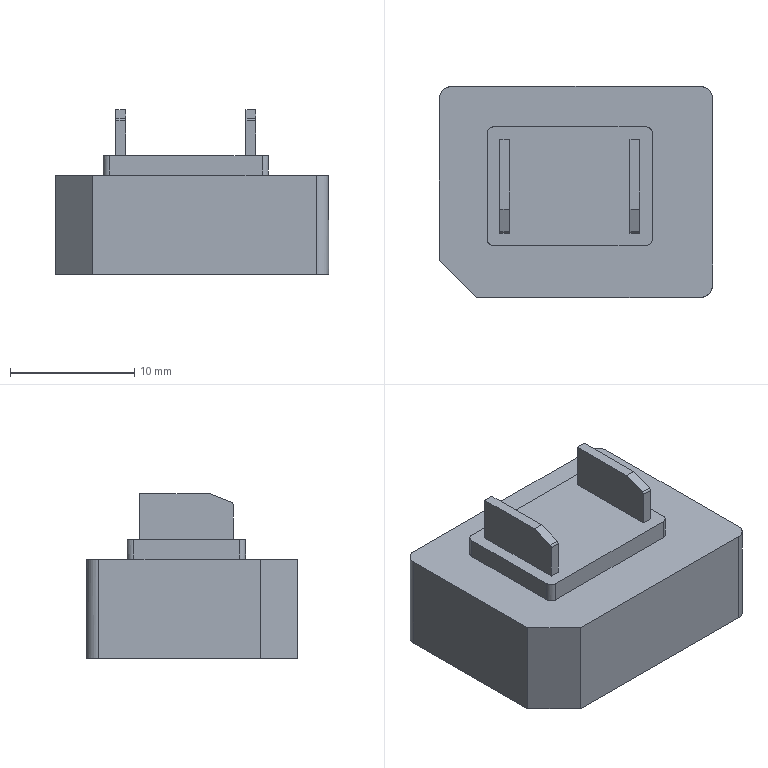NC program | PowerMill | posted by the shop | part box 22 x 17 x 13.286 mm
Lines 8691 to 10398 of 53717:
( TOOL ID   D3_1_1 )
( TOOL DIA. 3. TIP RAD 0 LENGTH 59.04 )
( Z = -3.934 )
T10 M6
T13
G91 G28 Z0
G0 G90 G54
M08
S18000 M3
X0 Y0 M8
G43 Z10.795 H10
X6.194 Y-3.121
Z1.037
G1 Z-.163 F960
X6.18 Y-3.08 F1600
X6.161 Y-3.04
X6.14 Y-3.002
X6.115 Y-2.966
X6.086 Y-2.932
X6.055 Y-2.902
X6.021 Y-2.874
X5.985 Y-2.849
X5.947 Y-2.828
X5.907 Y-2.811
X5.865 Y-2.797
X5.823 Y-2.787
X5.779 Y-2.781
X5.736 Y-2.779
X5.692 Y-2.78
X5.649 Y-2.786
X5.606 Y-2.796
X5.596 Y-2.799
X5.519 Y-2.822
X5.445 Y-2.84
X5.375 Y-2.854
X5.309 Y-2.863
X5.244 Y-2.868
X5.182 Y-2.87
X4.846 Y-2.871
X4.548 Y-2.87
X4.399 Y-2.871
X4.313 Y-2.87
X4.232 Y-2.866
X4.154 Y-2.858
X4.081 Y-2.846
X4.01 Y-2.832
X3.941 Y-2.813
X3.868 Y-2.79
X3.797 Y-2.763
X3.728 Y-2.733
X3.66 Y-2.699
X3.595 Y-2.661
X3.531 Y-2.62
X3.469 Y-2.575
X3.41 Y-2.528
X3.353 Y-2.477
X3.299 Y-2.424
X3.248 Y-2.367
X3.2 Y-2.308
X3.155 Y-2.247
X3.114 Y-2.183
X3.076 Y-2.118
X3.041 Y-2.05
X3.01 Y-1.981
X2.983 Y-1.911
X2.96 Y-1.84
X2.94 Y-1.768
X2.925 Y-1.695
X2.912 Y-1.62
X2.904 Y-1.544
X2.9 Y-1.466
X2.899 Y-1.393
X2.902 Y-1.317
X2.908 Y-1.241
X2.919 Y-1.165
X2.934 Y-1.09
X2.952 Y-1.017
X2.975 Y-.944
X3.001 Y-.872
X3.031 Y-.802
X3.064 Y-.734
X3.101 Y-.668
X3.141 Y-.604
X3.185 Y-.542
X3.231 Y-.483
X3.281 Y-.426
X3.334 Y-.372
X3.39 Y-.32
X3.449 Y-.271
X3.51 Y-.225
X3.572 Y-.183
X3.637 Y-.145
X3.704 Y-.11
X3.773 Y-.077
X3.844 Y-.049
X3.916 Y-.025
X3.988 Y-.004
X4.061 Y.012
X4.134 Y.025
X4.207 Y.033
X4.281 Y.038
X4.354 Y.039
X4.54 Y.04
X4.873
X5.099
X5.173 Y.039
X5.251 Y.035
X5.327 Y.028
X5.399 Y.018
X5.47 Y.004
X5.538 Y-.013
X5.607 Y-.034
X5.676 Y-.06
X5.745 Y-.089
X5.814 Y-.123
X5.881 Y-.16
X5.946 Y-.201
X6.009 Y-.245
X6.069 Y-.291
X6.126 Y-.34
X6.179 Y-.391
X6.228 Y-.445
X6.277 Y-.503
X6.323 Y-.564
X6.365 Y-.627
X6.405 Y-.692
X6.44 Y-.759
X6.473 Y-.828
X6.501 Y-.899
X6.526 Y-.971
X6.547 Y-1.044
X6.564 Y-1.119
X6.578 Y-1.194
X6.587 Y-1.27
X6.592 Y-1.346
X6.594 Y-1.422
X6.591 Y-1.5
X6.585 Y-1.578
X6.575 Y-1.654
X6.561 Y-1.729
X6.543 Y-1.803
X6.521 Y-1.876
X6.495 Y-1.948
X6.466 Y-2.017
X6.434 Y-2.085
X6.397 Y-2.152
X6.358 Y-2.216
X6.314 Y-2.279
X6.268 Y-2.339
X6.219 Y-2.396
X6.166 Y-2.451
X6.111 Y-2.503
X6.053 Y-2.552
X5.993 Y-2.598
X5.93 Y-2.641
X5.865 Y-2.68
X5.799 Y-2.716
X5.73 Y-2.748
X5.66 Y-2.776
X5.596 Y-2.799
X5.556 Y-2.815
X5.517 Y-2.835
X5.48 Y-2.859
X5.445 Y-2.885
X5.413 Y-2.915
X5.384 Y-2.948
X5.358 Y-2.983
X5.335 Y-3.02
X5.315 Y-3.059
X5.3 Y-3.1
X5.288 Y-3.142
X5.28 Y-3.185
X5.276 Y-3.229
X5.275 Y-3.272
X5.279 Y-3.316
X5.287 Y-3.359
X5.299 Y-3.401
X5.302 Y-3.41
X6.224 Y-3.172 Z-.193
X6.209 Y-3.131
X6.19 Y-3.092
X6.167 Y-3.055
X6.141 Y-3.019
X6.112 Y-2.987
X6.08 Y-2.957
X6.045 Y-2.93
X6.008 Y-2.906
X5.97 Y-2.886
X5.929 Y-2.87
X5.887 Y-2.857
X5.844 Y-2.848
X5.801 Y-2.843
X5.757 Y-2.842
X5.714 Y-2.845
X5.67 Y-2.852
X5.628 Y-2.863
X5.619 Y-2.866
X5.568 Y-2.883
X5.51 Y-2.899
X5.459 Y-2.911
X5.406 Y-2.922
X5.354 Y-2.93
X5.278 Y-2.938
X5.195 Y-2.944
X5.104 Y-2.945
X5.005
X4.637
X4.399 Y-2.946
X4.316 Y-2.945
X4.235 Y-2.941
X4.156 Y-2.933
X4.08 Y-2.921
X4.006 Y-2.905
X3.934 Y-2.886
X3.863 Y-2.863
X3.794 Y-2.837
X3.727 Y-2.807
X3.661 Y-2.774
X3.595 Y-2.736
X3.53 Y-2.694
X3.468 Y-2.65
X3.409 Y-2.602
X3.352 Y-2.551
X3.299 Y-2.498
X3.248 Y-2.442
X3.201 Y-2.384
X3.156 Y-2.322
X3.114 Y-2.259
X3.076 Y-2.193
X3.042 Y-2.126
X3.011 Y-2.058
X2.988 Y-1.998
X2.967 Y-1.937
X2.948 Y-1.875
X2.933 Y-1.811
X2.92 Y-1.742
X2.91 Y-1.669
X2.903 Y-1.592
X2.9 Y-1.515
X2.899 Y-1.441
X2.9 Y-1.366
X2.904 Y-1.289
X2.912 Y-1.212
X2.924 Y-1.137
X2.94 Y-1.063
X2.96 Y-.99
X2.983 Y-.919
X3.01 Y-.85
X3.041 Y-.78
X3.076 Y-.712
X3.114 Y-.646
X3.156 Y-.583
X3.201 Y-.521
X3.249 Y-.463
X3.3 Y-.406
X3.354 Y-.353
X3.41 Y-.302
X3.47 Y-.255
X3.531 Y-.21
X3.595 Y-.169
X3.661 Y-.131
X3.729 Y-.097
X3.799 Y-.067
X3.87 Y-.04
X3.942 Y-.017
X4.007 Y0
X4.082 Y.016
X4.153 Y.028
X4.22 Y.035
X4.284 Y.039
X4.347
X4.699 Y.04
X4.921 Y.041
X5.096
X5.198 Y.039
X5.27 Y.035
X5.342 Y.027
X5.415 Y.016
X5.488 Y0
X5.561 Y-.02
X5.633 Y-.044
X5.706 Y-.073
X5.774 Y-.103
X5.84 Y-.137
X5.905 Y-.174
X5.968 Y-.215
X6.029 Y-.26
X6.088 Y-.308
X6.145 Y-.359
X6.198 Y-.412
X6.248 Y-.468
X6.296 Y-.527
X6.34 Y-.588
X6.381 Y-.652
X6.419 Y-.718
X6.454 Y-.787
X6.485 Y-.857
X6.511 Y-.926
X6.534 Y-.996
X6.553 Y-1.068
X6.569 Y-1.142
X6.581 Y-1.218
X6.589 Y-1.295
X6.593 Y-1.373
X6.594 Y-1.443
X6.593 Y-1.514
X6.59 Y-1.586
X6.584 Y-1.661
X6.575 Y-1.733
X6.562 Y-1.801
X6.547 Y-1.864
X6.53 Y-1.924
X6.51 Y-1.984
X6.487 Y-2.044
X6.457 Y-2.113
X6.423 Y-2.181
X6.386 Y-2.246
X6.345 Y-2.31
X6.301 Y-2.372
X6.253 Y-2.431
X6.203 Y-2.488
X6.149 Y-2.542
X6.093 Y-2.593
X6.034 Y-2.642
X5.973 Y-2.687
X5.909 Y-2.729
X5.844 Y-2.767
X5.777 Y-2.802
X5.708 Y-2.832
X5.639 Y-2.86
X5.619 Y-2.866
X5.578 Y-2.882
X5.538 Y-2.901
X5.501 Y-2.924
X5.466 Y-2.95
X5.433 Y-2.979
X5.403 Y-3.011
X5.376 Y-3.045
X5.353 Y-3.082
X5.333 Y-3.121
X5.316 Y-3.162
X5.303 Y-3.203
X5.295 Y-3.246
X5.29 Y-3.29
X5.289 Y-3.333
X5.292 Y-3.377
X5.299 Y-3.42
X5.309 Y-3.463
X5.312 Y-3.472
X6.265 Y-3.206 Z-.223
X6.248 Y-3.166
X6.226 Y-3.128
X6.202 Y-3.092
X6.174 Y-3.058
X6.143 Y-3.027
X6.11 Y-2.999
X6.074 Y-2.974
X6.036 Y-2.952
X5.996 Y-2.934
X5.954 Y-2.92
X5.912 Y-2.909
X5.869 Y-2.902
X5.825 Y-2.9
X5.781 Y-2.901
X5.738 Y-2.906
X5.695 Y-2.916
X5.653 Y-2.929
X5.644 Y-2.932
X5.635 Y-2.936
X5.562 Y-2.96
X5.489 Y-2.979
X5.415 Y-2.995
X5.394 Y-2.999
X5.323 Y-3.009
X5.248 Y-3.016
X5.168 Y-3.02
X5.08
X4.878
X4.612
X4.417
X4.326
X4.246 Y-3.017
X4.173 Y-3.01
X4.106 Y-3.001
X4.04 Y-2.988
X3.965 Y-2.969
X3.892 Y-2.947
X3.821 Y-2.922
X3.751 Y-2.893
X3.683 Y-2.86
X3.616 Y-2.823
X3.552 Y-2.783
X3.489 Y-2.74
X3.429 Y-2.694
X3.372 Y-2.644
X3.317 Y-2.591
X3.265 Y-2.536
X3.216 Y-2.478
X3.17 Y-2.417
X3.127 Y-2.354
X3.088 Y-2.289
X3.052 Y-2.222
X3.02 Y-2.154
X2.991 Y-2.083
X2.966 Y-2.011
X2.945 Y-1.938
X2.928 Y-1.865
X2.915 Y-1.791
X2.906 Y-1.716
X2.901 Y-1.642
X2.899 Y-1.567
Y-1.393
X2.902 Y-1.317
X2.908 Y-1.242
X2.919 Y-1.166
X2.933 Y-1.092
X2.952 Y-1.018
X2.974 Y-.946
X3. Y-.875
X3.03 Y-.805
X3.063 Y-.736
X3.1 Y-.67
X3.14 Y-.606
X3.184 Y-.544
X3.231 Y-.484
X3.28 Y-.427
X3.333 Y-.372
X3.389 Y-.321
X3.447 Y-.272
X3.508 Y-.227
X3.571 Y-.184
X3.636 Y-.145
X3.703 Y-.11
X3.772 Y-.078
X3.843 Y-.05
X3.915 Y-.025
X3.988 Y-.005
X4.055 Y.011
X4.123 Y.023
X4.193 Y.031
X4.27 Y.037
X4.347 Y.04
X4.421
X4.799
X5.021
X5.173 Y.039
X5.247 Y.036
X5.32 Y.03
X5.394 Y.019
X5.467 Y.005
X5.54 Y-.014
X5.612 Y-.036
X5.683 Y-.063
X5.753 Y-.093
X5.822 Y-.127
X5.888 Y-.164
X5.952 Y-.204
X6.014 Y-.248
X6.074 Y-.295
X6.131 Y-.346
X6.185 Y-.399
X6.236 Y-.455
X6.285 Y-.513
X6.33 Y-.574
X6.372 Y-.637
X6.411 Y-.703
X6.446 Y-.77
X6.478 Y-.839
X6.506 Y-.91
X6.53 Y-.982
X6.55 Y-1.055
X6.567 Y-1.129
X6.579 Y-1.204
X6.588 Y-1.28
X6.592 Y-1.355
X6.593 Y-1.423
X6.594 Y-1.491
X6.593 Y-1.565
X6.591 Y-1.648
X6.586 Y-1.722
X6.578 Y-1.787
X6.568 Y-1.846
X6.556 Y-1.903
X6.541 Y-1.96
X6.524 Y-2.016
X6.504 Y-2.072
X6.483 Y-2.127
X6.454 Y-2.194
X6.421 Y-2.26
X6.384 Y-2.325
X6.343 Y-2.388
X6.299 Y-2.449
X6.251 Y-2.509
X6.2 Y-2.566
X6.147 Y-2.619
X6.091 Y-2.67
X6.033 Y-2.718
X5.972 Y-2.762
X5.908 Y-2.804
X5.843 Y-2.842
X5.775 Y-2.877
X5.706 Y-2.908
X5.644 Y-2.932
X5.604 Y-2.95
X5.566 Y-2.971
X5.53 Y-2.996
X5.496 Y-3.023
X5.465 Y-3.054
X5.437 Y-3.088
X5.412 Y-3.124
X5.39 Y-3.162
X5.372 Y-3.202
X5.358 Y-3.243
X5.347 Y-3.285
X5.34 Y-3.329
X5.338 Y-3.372
X5.339 Y-3.416
X5.344 Y-3.459
X5.354 Y-3.502
X5.367 Y-3.544
X5.37 Y-3.553
X6.291 Y-3.27 Z-.252
X6.274 Y-3.23
X6.252 Y-3.192
X6.228 Y-3.155
X6.2 Y-3.122
X6.169 Y-3.091
X6.135 Y-3.063
X6.099 Y-3.038
X6.061 Y-3.016
X6.021 Y-2.998
X5.98 Y-2.984
X5.937 Y-2.974
X5.894 Y-2.967
X5.85 Y-2.965
X5.807 Y-2.966
X5.763 Y-2.971
X5.721 Y-2.981
X5.679 Y-2.994
X5.67 Y-2.997
X5.665 Y-2.999
X5.59 Y-3.026
X5.517 Y-3.048
X5.445 Y-3.065
X5.376 Y-3.079
X5.308 Y-3.088
X5.242 Y-3.093
X5.176 Y-3.094
X4.849 Y-3.095
X4.572
X4.399 Y-3.096
X4.317 Y-3.095
X4.237 Y-3.091
X4.16 Y-3.083
X4.085 Y-3.072
X4.012 Y-3.057
X3.942 Y-3.038
X3.872 Y-3.016
X3.804 Y-2.99
X3.734 Y-2.96
X3.666 Y-2.926
X3.6 Y-2.889
X3.536 Y-2.848
X3.474 Y-2.804
X3.415 Y-2.757
X3.358 Y-2.706
X3.304 Y-2.653
X3.253 Y-2.597
X3.204 Y-2.538
X3.159 Y-2.477
X3.117 Y-2.414
X3.079 Y-2.349
X3.044 Y-2.281
X3.013 Y-2.212
X2.985 Y-2.141
X2.961 Y-2.069
X2.941 Y-1.996
X2.925 Y-1.922
X2.913 Y-1.847
X2.904 Y-1.772
X2.9 Y-1.696
X2.899 Y-1.621
Y-1.411
X2.901 Y-1.335
X2.907 Y-1.259
X2.916 Y-1.184
X2.93 Y-1.109
X2.947 Y-1.035
X2.969 Y-.962
X2.994 Y-.89
X3.023 Y-.82
X3.055 Y-.751
X3.092 Y-.685
X3.131 Y-.62
X3.174 Y-.557
X3.22 Y-.497
X3.269 Y-.439
X3.322 Y-.384
X3.377 Y-.332
X3.434 Y-.282
X3.495 Y-.236
X3.557 Y-.193
X3.622 Y-.153
X3.689 Y-.117
X3.758 Y-.085
X3.828 Y-.056
X3.899 Y-.03
X3.972 Y-.009
X4.039 Y.007
X4.106 Y.02
X4.174 Y.029
X4.249 Y.036
X4.328 Y.039
X4.399 Y.04
X4.799
X5. Y.041
X5.14 Y.04
X5.214 Y.039
X5.287 Y.033
X5.361 Y.024
X5.435 Y.011
X5.508 Y-.006
X5.581 Y-.027
X5.653 Y-.052
X5.725 Y-.08
X5.793 Y-.112
X5.86 Y-.147
X5.924 Y-.186
X5.987 Y-.228
X6.048 Y-.274
X6.106 Y-.323
X6.161 Y-.375
X6.214 Y-.429
X6.264 Y-.487
X6.31 Y-.546
X6.354 Y-.609
X6.394 Y-.673
X6.431 Y-.74
X6.464 Y-.808
X6.494 Y-.878
X6.519 Y-.95
X6.542 Y-1.022
X6.56 Y-1.096
X6.574 Y-1.17
X6.584 Y-1.246
X6.591 Y-1.321
X6.593 Y-1.397
Y-1.473
Y-1.633
X6.591 Y-1.706
X6.587 Y-1.78
X6.579 Y-1.854
X6.566 Y-1.927
X6.55 Y-2.
X6.53 Y-2.073
X6.506 Y-2.144
X6.478 Y-2.215
X6.446 Y-2.285
X6.411 Y-2.352
X6.373 Y-2.417
X6.331 Y-2.48
X6.286 Y-2.541
X6.237 Y-2.599
X6.186 Y-2.655
X6.132 Y-2.709
X6.075 Y-2.759
X6.015 Y-2.806
X5.953 Y-2.85
X5.889 Y-2.89
X5.823 Y-2.928
X5.755 Y-2.961
X5.686 Y-2.991
X5.67 Y-2.997
X5.63 Y-3.015
X5.591 Y-3.036
X5.555 Y-3.061
X5.522 Y-3.089
X5.491 Y-3.12
X5.463 Y-3.154
X5.438 Y-3.19
X5.416 Y-3.228
X5.398 Y-3.268
X5.384 Y-3.309
X5.373 Y-3.351
X5.367 Y-3.395
X5.364 Y-3.438
X5.366 Y-3.482
X5.371 Y-3.526
X5.381 Y-3.568
X5.394 Y-3.61
X5.397 Y-3.619
X6.326 Y-3.316 Z-.282
X6.307 Y-3.277
X6.284 Y-3.239
X6.259 Y-3.204
X6.23 Y-3.171
X6.198 Y-3.141
X6.164 Y-3.113
X6.127 Y-3.09
X6.088 Y-3.069
X6.048 Y-3.052
X6.006 Y-3.039
X5.964 Y-3.03
X5.92 Y-3.025
X5.876 Y-3.023
X5.833 Y-3.026
X5.789 Y-3.032
X5.747 Y-3.043
X5.706 Y-3.057
X5.697 Y-3.061
X5.678 Y-3.069
X5.607 Y-3.095
X5.595 Y-3.099
X5.517 Y-3.122
X5.443 Y-3.14
X5.373 Y-3.154
X5.307 Y-3.163
X5.243 Y-3.168
X5.18 Y-3.169
X4.845 Y-3.17
X4.52
X4.399
X4.31 Y-3.169
X4.23 Y-3.165
X4.157 Y-3.158
X4.088 Y-3.147
X4.013 Y-3.131
X3.939 Y-3.112
X3.866 Y-3.089
X3.795 Y-3.062
X3.726 Y-3.031
X3.659 Y-2.997
X3.593 Y-2.959
X3.529 Y-2.918
X3.468 Y-2.874
X3.409 Y-2.826
X3.352 Y-2.775
X3.298 Y-2.722
X3.247 Y-2.666
X3.199 Y-2.607
X3.155 Y-2.545
X3.113 Y-2.482
X3.075 Y-2.416
X3.041 Y-2.349
X3.01 Y-2.279
X2.982 Y-2.208
X2.959 Y-2.136
X2.939 Y-2.063
X2.923 Y-1.989
X2.912 Y-1.915
X2.904 Y-1.84
X2.9 Y-1.765
X2.899 Y-1.69
Y-1.193
Y-.349
Y2.899
Y4.199
X2.901 Y4.285
X2.906 Y4.363
X2.914 Y4.435
X2.925 Y4.502
X2.942 Y4.577
X2.962 Y4.651
X2.986 Y4.723
X3.014 Y4.794
X3.046 Y4.863
X3.081 Y4.931
X3.12 Y4.996
X3.162 Y5.06
X3.207 Y5.121
X3.255 Y5.179
X3.307 Y5.235
X3.361 Y5.288
X3.417 Y5.338
X3.476 Y5.384
X3.538 Y5.428
X3.603 Y5.469
X3.669 Y5.506
X3.737 Y5.54
X3.806 Y5.57
X3.877 Y5.596
X3.948 Y5.619
X4.021 Y5.638
X4.094 Y5.652
X4.167 Y5.663
X4.238 Y5.67
X4.31 Y5.672
X4.495 Y5.674
X4.699
X5.007
X5.099
X5.185 Y5.673
X5.265 Y5.669
X5.339 Y5.661
X5.409 Y5.65
X5.484 Y5.634
X5.557 Y5.615
X5.63 Y5.591
X5.7 Y5.564
X5.77 Y5.533
X5.837 Y5.499
X5.903 Y5.461
X5.967 Y5.419
X6.028 Y5.375
X6.087 Y5.327
X6.144 Y5.276
X6.197 Y5.222
X6.248 Y5.166
X6.296 Y5.107
X6.34 Y5.045
X6.381 Y4.982
X6.419 Y4.916
X6.454 Y4.847
X6.485 Y4.777
X6.511 Y4.709
X6.534 Y4.64
X6.552 Y4.57
X6.568 Y4.497
X6.579 Y4.422
X6.587 Y4.344
X6.592 Y4.262
X6.593 Y4.177
Y2.28
Y-1.3
X6.594 Y-1.699
X6.592 Y-1.778
X6.587 Y-1.857
X6.577 Y-1.934
X6.564 Y-2.01
X6.547 Y-2.085
X6.526 Y-2.158
X6.501 Y-2.23
X6.473 Y-2.3
X6.442 Y-2.369
X6.406 Y-2.435
X6.368 Y-2.499
X6.326 Y-2.562
X6.28 Y-2.623
X6.231 Y-2.681
X6.18 Y-2.737
X6.125 Y-2.79
X6.068 Y-2.839
X6.008 Y-2.886
X5.946 Y-2.93
X5.882 Y-2.97
X5.816 Y-3.006
X5.748 Y-3.039
X5.697 Y-3.061
X5.657 Y-3.08
X5.619 Y-3.102
X5.584 Y-3.128
X5.551 Y-3.157
X5.521 Y-3.189
X5.494 Y-3.223
X5.47 Y-3.26
X5.449 Y-3.298
X5.433 Y-3.339
X5.419 Y-3.38
X5.41 Y-3.423
X5.405 Y-3.467
X5.404 Y-3.51
X5.406 Y-3.554
X5.413 Y-3.597
X5.423 Y-3.64
X5.438 Y-3.681
X5.441 Y-3.69
X6.349 Y-3.388 Z-.312
X6.33 Y-3.348
X6.309 Y-3.31
X6.283 Y-3.275
X6.255 Y-3.241
X6.223 Y-3.211
X6.189 Y-3.183
X6.153 Y-3.159
X6.115 Y-3.138
X6.074 Y-3.121
X6.033 Y-3.107
X5.99 Y-3.097
X5.947 Y-3.091
X5.903 Y-3.09
X5.859 Y-3.092
X5.816 Y-3.098
X5.774 Y-3.108
X5.732 Y-3.122
X5.723 Y-3.125
X5.661 Y-3.15
X5.591 Y-3.175
X5.52 Y-3.195
X5.508 Y-3.199
X5.428 Y-3.217
X5.357 Y-3.23
X5.292 Y-3.239
X5.231 Y-3.243
X5.172 Y-3.244
X4.425 Y-3.245
X4.367
X4.309 Y-3.244
X4.251 Y-3.241
X4.193 Y-3.237
X4.135 Y-3.23
X4.076 Y-3.219
X4.019 Y-3.207
X3.963 Y-3.193
X3.896 Y-3.174
X3.828 Y-3.15
X3.759 Y-3.121
X3.69 Y-3.088
X3.623 Y-3.052
X3.558 Y-3.012
X3.495 Y-2.969
X3.435 Y-2.923
X3.377 Y-2.873
X3.322 Y-2.821
X3.27 Y-2.766
X3.221 Y-2.709
X3.176 Y-2.65
X3.133 Y-2.587
X3.093 Y-2.522
X3.056 Y-2.455
X3.024 Y-2.387
X2.995 Y-2.317
X2.969 Y-2.245
X2.948 Y-2.173
X2.93 Y-2.099
X2.917 Y-2.025
X2.907 Y-1.95
X2.901 Y-1.875
X2.9 Y-1.8
X2.899 Y-1.317
Y-.472
Y2.899
Y4.199
X2.901 Y4.285
X2.906 Y4.363
X2.914 Y4.435
X2.925 Y4.502
X2.942 Y4.577
X2.962 Y4.651
X2.986 Y4.723
X3.014 Y4.794
X3.046 Y4.863
X3.081 Y4.931
X3.12 Y4.996
X3.162 Y5.06
X3.207 Y5.121
X3.255 Y5.179
X3.307 Y5.235
X3.361 Y5.288
X3.417 Y5.338
X3.476 Y5.384
X3.538 Y5.428
X3.603 Y5.469
X3.669 Y5.506
X3.737 Y5.54
X3.806 Y5.57
X3.877 Y5.596
X3.948 Y5.619
X4.021 Y5.638
X4.094 Y5.652
X4.167 Y5.663
X4.238 Y5.67
X4.31 Y5.672
X4.495 Y5.674
X4.699
X5.007
X5.099
X5.185 Y5.673
X5.265 Y5.669
X5.339 Y5.661
X5.409 Y5.65
X5.484 Y5.634
X5.557 Y5.615
X5.63 Y5.591
X5.7 Y5.564
X5.77 Y5.533
X5.837 Y5.499
X5.903 Y5.461
X5.967 Y5.419
X6.028 Y5.375
X6.087 Y5.327
X6.144 Y5.276
X6.197 Y5.222
X6.248 Y5.166
X6.296 Y5.107
X6.34 Y5.045
X6.381 Y4.982
X6.419 Y4.916
X6.454 Y4.847
X6.485 Y4.777
X6.511 Y4.709
X6.534 Y4.64
X6.552 Y4.57
X6.568 Y4.497
X6.579 Y4.422
X6.587 Y4.344
X6.592 Y4.262
X6.593 Y4.177
Y2.28
Y-1.3
Y-1.799
X6.591 Y-1.875
X6.585 Y-1.951
X6.575 Y-2.027
X6.561 Y-2.101
X6.543 Y-2.175
X6.522 Y-2.248
X6.496 Y-2.32
X6.467 Y-2.39
X6.434 Y-2.458
X6.398 Y-2.525
X6.358 Y-2.589
X6.315 Y-2.652
X6.269 Y-2.712
X6.219 Y-2.77
X6.167 Y-2.825
X6.111 Y-2.877
X6.054 Y-2.926
X5.993 Y-2.972
X5.931 Y-3.014
X5.866 Y-3.054
X5.799 Y-3.09
X5.731 Y-3.122
X5.723 Y-3.125
X5.683 Y-3.144
X5.645 Y-3.166
X5.61 Y-3.191
X5.576 Y-3.219
X5.546 Y-3.251
X5.518 Y-3.285
X5.494 Y-3.321
X5.473 Y-3.36
X5.456 Y-3.4
X5.442 Y-3.441
X5.432 Y-3.484
X5.427 Y-3.527
X5.425 Y-3.571
X5.427 Y-3.615
X5.433 Y-3.658
X5.443 Y-3.701
X5.457 Y-3.742
X5.46 Y-3.751
X6.395 Y-3.408 Z-.342
X6.374 Y-3.369
X6.349 Y-3.333
X6.322 Y-3.299
X6.291 Y-3.268
X6.258 Y-3.239
X6.222 Y-3.214
X6.184 Y-3.192
X6.145 Y-3.174
X6.103 Y-3.159
X6.061 Y-3.148
X6.018 Y-3.141
X5.974 Y-3.138
X5.93 Y-3.139
X5.887 Y-3.144
X5.844 Y-3.153
X5.802 Y-3.166
X5.762 Y-3.182
X5.753 Y-3.187
X5.747 Y-3.189
X5.677 Y-3.219
X5.605 Y-3.245
X5.533 Y-3.267
X5.459 Y-3.286
X5.39 Y-3.299
X5.323 Y-3.309
X5.249 Y-3.316
X5.167 Y-3.319
X5.098 Y-3.32
X4.679 Y-3.319
X4.399 Y-3.321
X4.316 Y-3.32
X4.237 Y-3.315
X4.159 Y-3.307
X4.084 Y-3.296
X4.01 Y-3.28
X3.939 Y-3.261
X3.869 Y-3.239
X3.801 Y-3.213
X3.733 Y-3.184
X3.665 Y-3.15
X3.599 Y-3.113
X3.535 Y-3.072
X3.474 Y-3.028
X3.414 Y-2.981
X3.358 Y-2.93
X3.303 Y-2.877
X3.252 Y-2.821
X3.204 Y-2.762
X3.159 Y-2.701
X3.117 Y-2.638
X3.079 Y-2.572
X3.044 Y-2.505
X3.013 Y-2.436
X2.985 Y-2.366
X2.961 Y-2.293
X2.941 Y-2.219
X2.925 Y-2.145
X2.912 Y-2.071
X2.904 Y-1.997
X2.9 Y-1.922
X2.899 Y-1.848
Y-1.408
Y-.799
Y2.899
Y4.199
X2.901 Y4.285
X2.906 Y4.363
X2.914 Y4.435
X2.925 Y4.502
X2.942 Y4.577
X2.962 Y4.651
X2.986 Y4.723
X3.014 Y4.794
X3.046 Y4.863
X3.081 Y4.931
X3.12 Y4.996
X3.162 Y5.06
X3.207 Y5.121
X3.255 Y5.179
X3.307 Y5.235
X3.361 Y5.288
X3.417 Y5.338
X3.476 Y5.384
X3.538 Y5.428
X3.603 Y5.469
X3.669 Y5.506
X3.737 Y5.54
X3.806 Y5.57
X3.877 Y5.596
X3.948 Y5.619
X4.021 Y5.638
X4.094 Y5.652
X4.167 Y5.663
X4.238 Y5.67
X4.31 Y5.672
X4.495 Y5.674
X4.699
X5.007
X5.099
X5.185 Y5.673
X5.265 Y5.669
X5.339 Y5.661
X5.409 Y5.65
X5.484 Y5.634
X5.557 Y5.615
X5.63 Y5.591
X5.7 Y5.564
X5.77 Y5.533
X5.837 Y5.499
X5.903 Y5.461
X5.967 Y5.419
X6.028 Y5.375
X6.087 Y5.327
X6.144 Y5.276
X6.197 Y5.222
X6.248 Y5.166
X6.296 Y5.107
X6.34 Y5.045
X6.381 Y4.982
X6.419 Y4.916
X6.454 Y4.847
X6.485 Y4.777
X6.511 Y4.709
X6.534 Y4.64
X6.552 Y4.57
X6.568 Y4.497
X6.579 Y4.422
X6.587 Y4.344
X6.592 Y4.262
X6.593 Y4.177
Y2.28
Y-1.3
X6.594 Y-1.699
Y-1.799
X6.593 Y-1.88
X6.59 Y-1.961
X6.583 Y-2.04
X6.573 Y-2.115
X6.559 Y-2.186
X6.543 Y-2.254
X6.523 Y-2.32
X6.501 Y-2.383
X6.475 Y-2.447
X6.443 Y-2.516
X6.407 Y-2.584
X6.368 Y-2.649
X6.326 Y-2.712
X6.28 Y-2.773
X6.231 Y-2.831
X6.18 Y-2.886
X6.125 Y-2.939
X6.068 Y-2.989
X6.008 Y-3.035
X5.946 Y-3.079
X5.882 Y-3.119
X5.815 Y-3.156
X5.753 Y-3.187
X5.714 Y-3.208
X5.678 Y-3.232
X5.644 Y-3.26
X5.613 Y-3.29
X5.584 Y-3.323
X5.559 Y-3.359
X5.537 Y-3.397
X5.519 Y-3.437
X5.504 Y-3.478
X5.493 Y-3.52
X5.486 Y-3.563
X5.483 Y-3.607
X5.484 Y-3.651
X5.489 Y-3.694
X5.498 Y-3.737
X5.511 Y-3.779
X5.527 Y-3.82
X5.532 Y-3.828
X6.424 Y-3.467 Z-.372
X6.403 Y-3.429
X6.379 Y-3.393
X6.351 Y-3.359
X6.321 Y-3.327
X6.287 Y-3.299
X6.252 Y-3.274
X6.214 Y-3.252
X6.174 Y-3.234
X6.133 Y-3.219
X6.09 Y-3.208
X6.047 Y-3.201
X6.004 Y-3.198
X5.96 Y-3.199
X5.916 Y-3.204
X5.874 Y-3.213
X5.832 Y-3.226
X5.791 Y-3.243
X5.782 Y-3.247
X5.75 Y-3.263
X5.681 Y-3.292
X5.664 Y-3.299
X5.588 Y-3.326
X5.515 Y-3.348
X5.444 Y-3.365
X5.374 Y-3.378
X5.306 Y-3.387
X5.24 Y-3.392
X5.175 Y-3.393
X4.732 Y-3.394
X4.399
X4.305 Y-3.393
X4.223 Y-3.388
X4.149 Y-3.381
X4.079 Y-3.37
X4.008 Y-3.355
X3.937 Y-3.336
X3.865 Y-3.313
X3.794 Y-3.286
X3.725 Y-3.255
X3.657 Y-3.22
X3.591 Y-3.183
X3.527 Y-3.141
X3.466 Y-3.097
X3.407 Y-3.049
X3.35 Y-2.998
X3.297 Y-2.945
X3.246 Y-2.888
X3.198 Y-2.829
X3.153 Y-2.768
X3.112 Y-2.704
X3.074 Y-2.639
X3.04 Y-2.571
X3.009 Y-2.501
X2.981 Y-2.43
X2.958 Y-2.358
X2.939 Y-2.285
X2.923 Y-2.211
X2.911 Y-2.137
X2.904 Y-2.062
X2.9 Y-1.987
Y-1.912
X2.899 Y-1.319
Y-.307
Y2.899
Y4.199
X2.901 Y4.285
X2.906 Y4.363
X2.914 Y4.435
X2.925 Y4.502
X2.942 Y4.577
X2.962 Y4.651
X2.986 Y4.723
X3.014 Y4.794
X3.046 Y4.863
X3.081 Y4.931
X3.12 Y4.996
X3.162 Y5.059
X3.207 Y5.121
X3.255 Y5.179
X3.307 Y5.235
X3.361 Y5.288
X3.417 Y5.338
X3.476 Y5.384
X3.538 Y5.428
X3.602 Y5.469
X3.669 Y5.506
X3.737 Y5.54
X3.806 Y5.57
X3.876 Y5.596
X3.948 Y5.619
X4.021 Y5.637
X4.094 Y5.652
X4.166 Y5.663
X4.238 Y5.67
X4.31 Y5.672
X4.495 Y5.674
X4.699
X4.981
X5.099 Y5.675
X5.183 Y5.674
X5.264 Y5.669
X5.341 Y5.661
X5.415 Y5.649
X5.485 Y5.634
X5.555 Y5.615
X5.628 Y5.592
X5.699 Y5.565
X5.768 Y5.534
X5.836 Y5.5
X5.902 Y5.462
X5.965 Y5.421
X6.027 Y5.376
X6.086 Y5.328
X6.142 Y5.277
X6.196 Y5.224
X6.247 Y5.167
X6.295 Y5.108
X6.339 Y5.047
X6.38 Y4.984
X6.418 Y4.918
X6.453 Y4.849
X6.484 Y4.779
X6.511 Y4.711
X6.533 Y4.642
X6.552 Y4.572
X6.567 Y4.499
X6.579 Y4.424
X6.587 Y4.346
X6.592 Y4.265
X6.593 Y4.18
Y2.285
Y-1.3
X6.592 Y-1.596
Y-1.827
X6.593 Y-1.899
Y-1.968
X6.59 Y-2.036
X6.585 Y-2.105
X6.576 Y-2.175
X6.563 Y-2.246
X6.546 Y-2.317
X6.525 Y-2.387
X6.501 Y-2.455
X6.475 Y-2.523
X6.444 Y-2.59
X6.408 Y-2.656
X6.37 Y-2.721
X6.328 Y-2.784
X6.282 Y-2.845
X6.234 Y-2.903
X6.182 Y-2.959
X6.128 Y-3.012
X6.071 Y-3.062
X6.011 Y-3.109
X5.949 Y-3.152
X5.885 Y-3.193
X5.818 Y-3.229
X5.782 Y-3.247
X5.744 Y-3.268
X5.708 Y-3.293
X5.674 Y-3.32
X5.642 Y-3.351
X5.614 Y-3.384
X5.589 Y-3.42
X5.567 Y-3.458
X5.549 Y-3.497
X5.534 Y-3.539
X5.523 Y-3.581
X5.516 Y-3.624
X5.513 Y-3.668
X5.514 Y-3.712
X5.52 Y-3.755
X5.529 Y-3.798
X5.541 Y-3.84
X5.558 Y-3.88
X5.562 Y-3.889
X6.455 Y-3.524 Z-.402
X6.434 Y-3.486
X6.41 Y-3.45
X6.382 Y-3.416
X6.351 Y-3.385
X6.318 Y-3.357
X6.282 Y-3.332
X6.244 Y-3.31
X6.204 Y-3.292
X6.163 Y-3.277
X6.12 Y-3.267
X6.077 Y-3.26
X6.033 Y-3.257
X5.989 Y-3.259
X5.946 Y-3.264
X5.903 Y-3.273
X5.861 Y-3.286
X5.821 Y-3.303
X5.812 Y-3.307
X5.757 Y-3.334
X5.688 Y-3.364
X5.617 Y-3.39
X5.593 Y-3.399
X5.515 Y-3.422
X5.441 Y-3.44
X5.371 Y-3.453
X5.305 Y-3.462
X5.241 Y-3.467
X5.178 Y-3.468
X4.83 Y-3.469
X4.54
X4.399 Y-3.47
X4.313 Y-3.469
X4.232 Y-3.464
X4.155 Y-3.456
X4.081 Y-3.445
X4.011 Y-3.43
X3.941 Y-3.412
X3.869 Y-3.389
X3.797 Y-3.362
X3.728 Y-3.331
X3.66 Y-3.297
X3.594 Y-3.259
X3.531 Y-3.218
X3.469 Y-3.174
X3.41 Y-3.126
X3.353 Y-3.075
X3.299 Y-3.022
X3.248 Y-2.965
X3.2 Y-2.906
X3.155 Y-2.845
X3.113 Y-2.782
X3.075 Y-2.716
X3.041 Y-2.65
X3.011 Y-2.582
X2.984 Y-2.512
X2.961 Y-2.44
X2.941 Y-2.367
X2.925 Y-2.292
X2.913 Y-2.216
X2.904 Y-2.138
X2.9 Y-2.058
X2.899 Y-1.977
Y-.516
Y2.899
Y3.9
Y4.199
X2.9 Y4.282
X2.905 Y4.361
X2.914 Y4.436
X2.926 Y4.507
X2.943 Y4.581
X2.963 Y4.654
X2.987 Y4.726
X3.015 Y4.797
X3.047 Y4.866
X3.083 Y4.933
X3.121 Y4.999
X3.164 Y5.062
X3.209 Y5.123
X3.257 Y5.181
X3.309 Y5.237
X3.363 Y5.29
X3.42 Y5.34
X3.479 Y5.386
X3.54 Y5.43
X3.605 Y5.471
X3.672 Y5.508
X3.74 Y5.541
X3.809 Y5.571
X3.879 Y5.597
X3.951 Y5.619
X4.024 Y5.638
X4.097 Y5.653
X4.169 Y5.663
X4.241 Y5.67
X4.313 Y5.672
X4.499 Y5.674
X4.699
X4.981
X5.099 Y5.675
X5.183 Y5.674
X5.264 Y5.669
X5.341 Y5.661
X5.415 Y5.649
X5.485 Y5.634
X5.555 Y5.615
X5.628 Y5.592
X5.699 Y5.565
X5.768 Y5.534
X5.836 Y5.5
X5.902 Y5.462
X5.965 Y5.421
X6.027 Y5.376
X6.086 Y5.328
X6.142 Y5.277
X6.196 Y5.224
X6.247 Y5.167
X6.295 Y5.108
X6.339 Y5.047
X6.38 Y4.984
X6.418 Y4.918
X6.453 Y4.849
X6.484 Y4.779
X6.511 Y4.711
X6.533 Y4.642
X6.552 Y4.572
X6.567 Y4.499
X6.579 Y4.424
X6.587 Y4.346
X6.592 Y4.265
X6.593 Y4.18
Y2.285
Y-.86
X6.594 Y-1.999
X6.592 Y-2.077
X6.587 Y-2.154
X6.578 Y-2.229
X6.565 Y-2.304
X6.548 Y-2.379
X6.528 Y-2.452
X6.503 Y-2.525
X6.477 Y-2.593
X6.446 Y-2.66
X6.412 Y-2.725
X6.374 Y-2.79
X6.332 Y-2.853
X6.286 Y-2.914
X6.237 Y-2.973
X6.186 Y-3.029
X6.132 Y-3.082
X6.075 Y-3.132
X6.016 Y-3.179
X5.955 Y-3.223
X5.891 Y-3.264
X5.825 Y-3.301
X5.812 Y-3.307
X5.774 Y-3.328
X5.738 Y-3.353
X5.704 Y-3.381
X5.673 Y-3.412
X5.645 Y-3.445
X5.62 Y-3.481
X5.598 Y-3.519
X5.58 Y-3.559
X5.565 Y-3.6
X5.555 Y-3.643
X5.548 Y-3.686
X5.545 Y-3.73
X5.547 Y-3.773
X5.552 Y-3.817
X5.561 Y-3.859
X5.574 Y-3.901
X5.591 Y-3.942
X5.595 Y-3.951
X6.494 Y-3.56 Z-.432
X6.471 Y-3.522
X6.445 Y-3.487
X6.417 Y-3.454
X6.385 Y-3.424
X6.35 Y-3.397
X6.314 Y-3.373
X6.275 Y-3.353
X6.234 Y-3.336
X6.193 Y-3.323
X6.15 Y-3.314
X6.106 Y-3.309
X6.063 Y-3.308
X6.019 Y-3.31
X5.976 Y-3.317
X5.933 Y-3.328
X5.892 Y-3.342
X5.852 Y-3.361
X5.843 Y-3.365
X5.801 Y-3.388
X5.732 Y-3.421
X5.663 Y-3.449
X5.592 Y-3.474
X5.521 Y-3.495
X5.506 Y-3.499
X5.454 Y-3.511
X5.402 Y-3.522
X5.35 Y-3.529
X5.273 Y-3.537
X5.19 Y-3.542
X5.099 Y-3.544
X4.399
X4.305 Y-3.542
X4.222 Y-3.537
X4.145 Y-3.53
X4.074 Y-3.519
X4.008 Y-3.505
X3.943 Y-3.487
X3.87 Y-3.464
X3.798 Y-3.437
X3.729 Y-3.406
X3.66 Y-3.372
X3.594 Y-3.334
X3.53 Y-3.293
X3.469 Y-3.249
X3.41 Y-3.201
X3.353 Y-3.151
X3.299 Y-3.097
X3.248 Y-3.041
X3.2 Y-2.982
X3.156 Y-2.921
X3.114 Y-2.857
X3.076 Y-2.791
X3.041 Y-2.724
X3.01 Y-2.654
X2.983 Y-2.584
X2.959 Y-2.511
X2.939 Y-2.438
X2.923 Y-2.364
X2.912 Y-2.29
X2.904 Y-2.216
X2.9 Y-2.142
X2.899 Y-2.068
Y-1.387
Y2.899
Y4.199
X2.901 Y4.285
X2.906 Y4.363
X2.914 Y4.435
X2.925 Y4.502
X2.942 Y4.577
X2.962 Y4.651
X2.986 Y4.723
X3.014 Y4.794
X3.046 Y4.863
X3.081 Y4.931
X3.12 Y4.996
X3.162 Y5.059
X3.207 Y5.121
X3.255 Y5.179
X3.307 Y5.235
X3.361 Y5.288
X3.417 Y5.338
X3.476 Y5.384
X3.538 Y5.428
X3.602 Y5.469
X3.669 Y5.506
X3.737 Y5.54
X3.806 Y5.57
X3.876 Y5.596
X3.948 Y5.619
X4.021 Y5.637
X4.094 Y5.652
X4.166 Y5.663
X4.238 Y5.67
X4.31 Y5.672
X4.495 Y5.674
X4.699
X4.981
X5.099 Y5.675
X5.183 Y5.674
X5.264 Y5.669
X5.341 Y5.661
X5.415 Y5.649
X5.485 Y5.634
X5.555 Y5.615
X5.628 Y5.592
X5.699 Y5.565
X5.768 Y5.534
X5.836 Y5.5
X5.902 Y5.462
X5.965 Y5.421
X6.027 Y5.376
X6.086 Y5.328
X6.142 Y5.277
X6.196 Y5.224
X6.247 Y5.167
X6.295 Y5.108
X6.339 Y5.047
X6.38 Y4.984
X6.418 Y4.918
X6.453 Y4.849
X6.484 Y4.779
X6.511 Y4.711
X6.533 Y4.642
X6.552 Y4.572
X6.567 Y4.499
X6.579 Y4.424
X6.587 Y4.346
X6.592 Y4.265
X6.593 Y4.18
Y2.285
Y-1.3
Y-2.099
X6.591 Y-2.175
X6.585 Y-2.251
X6.575 Y-2.326
X6.561 Y-2.4
X6.544 Y-2.474